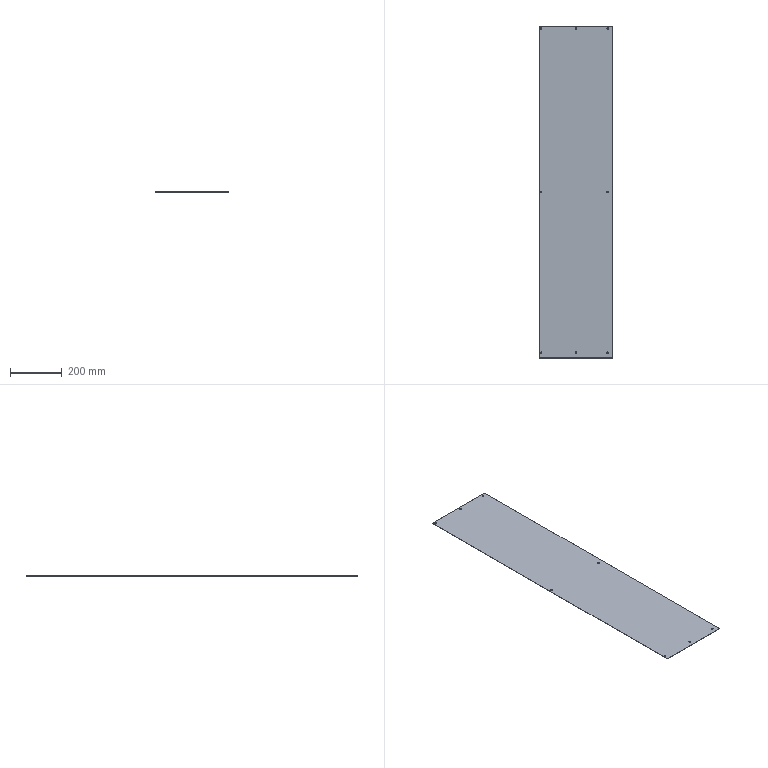Part | SolidWorks | features FlatPattern 1, HoleWzd 1, SMBaseFlange 1, SheetMetal 1 | 1 solid | 22 faces | box 285 x 1280 x 1.2 mm | volume 437432 mm3 | cylinder 16 | plane 6 | commonest cylinder face diameters 6.6 x16
STEP:
#1=CARTESIAN_POINT('',(-137.8,630.,-1.2));
#2=VERTEX_POINT('',#1);
#3=CARTESIAN_POINT('',(-131.2,630.,-1.2));
#4=VERTEX_POINT('',#3);
#5=CARTESIAN_POINT('',(-134.5,630.,-1.2));
#6=DIRECTION('',(0.,0.,1.));
#7=DIRECTION('',(1.,0.,0.));
#8=AXIS2_PLACEMENT_3D('',#5,#6,#7);
#9=CIRCLE('',#8,3.3);
#10=EDGE_CURVE('',#2,#4,#9,.T.);
#11=ORIENTED_EDGE('',*,*,#10,.F.);
#12=CARTESIAN_POINT('',(-137.8,630.,0.));
#13=VERTEX_POINT('',#12);
#14=CARTESIAN_POINT('',(-137.8,630.,0.));
#15=DIRECTION('',(0.,0.,1.));
#16=VECTOR('',#15,1000.);
#17=LINE('',#14,#16);
#18=EDGE_CURVE('',#2,#13,#17,.T.);
#19=ORIENTED_EDGE('',*,*,#18,.T.);
#20=CARTESIAN_POINT('',(-131.2,630.,0.));
#21=VERTEX_POINT('',#20);
#22=CARTESIAN_POINT('',(-134.5,630.,0.));
#23=DIRECTION('',(0.,0.,1.));
#24=DIRECTION('',(1.,0.,0.));
#25=AXIS2_PLACEMENT_3D('',#22,#23,#24);
#26=CIRCLE('',#25,3.3);
#27=EDGE_CURVE('',#13,#21,#26,.T.);
#28=ORIENTED_EDGE('',*,*,#27,.T.);
#29=CARTESIAN_POINT('',(-131.2,630.,0.));
#30=DIRECTION('',(0.,0.,1.));
#31=VECTOR('',#30,1000.);
#32=LINE('',#29,#31);
#33=EDGE_CURVE('',#4,#21,#32,.T.);
#34=ORIENTED_EDGE('',*,*,#33,.F.);
#35=EDGE_LOOP('',(#11,#19,#28,#34));
#36=FACE_OUTER_BOUND('',#35,.T.);
#37=CARTESIAN_POINT('',(-134.5,630.,0.));
#38=DIRECTION('',(0.,0.,1.));
#39=DIRECTION('',(1.,0.,0.));
#40=AXIS2_PLACEMENT_3D('',#37,#38,#39);
#41=CYLINDRICAL_SURFACE('',#40,3.3);
#42=ADVANCED_FACE('',(#36),#41,.F.);
#43=CARTESIAN_POINT('',(-137.8,0.,-1.2));
#44=VERTEX_POINT('',#43);
#45=CARTESIAN_POINT('',(-131.2,0.,-1.2));
#46=VERTEX_POINT('',#45);
#47=CARTESIAN_POINT('',(-134.5,0.,-1.2));
#48=DIRECTION('',(0.,0.,1.));
#49=DIRECTION('',(1.,0.,0.));
#50=AXIS2_PLACEMENT_3D('',#47,#48,#49);
#51=CIRCLE('',#50,3.3);
#52=EDGE_CURVE('',#44,#46,#51,.T.);
#53=ORIENTED_EDGE('',*,*,#52,.F.);
#54=CARTESIAN_POINT('',(-137.8,0.,0.));
#55=VERTEX_POINT('',#54);
#56=CARTESIAN_POINT('',(-137.8,0.,0.));
#57=DIRECTION('',(0.,0.,1.));
#58=VECTOR('',#57,1000.);
#59=LINE('',#56,#58);
#60=EDGE_CURVE('',#44,#55,#59,.T.);
#61=ORIENTED_EDGE('',*,*,#60,.T.);
#62=CARTESIAN_POINT('',(-131.2,0.,0.));
#63=VERTEX_POINT('',#62);
#64=CARTESIAN_POINT('',(-134.5,0.,0.));
#65=DIRECTION('',(0.,0.,1.));
#66=DIRECTION('',(1.,0.,0.));
#67=AXIS2_PLACEMENT_3D('',#64,#65,#66);
#68=CIRCLE('',#67,3.3);
#69=EDGE_CURVE('',#55,#63,#68,.T.);
#70=ORIENTED_EDGE('',*,*,#69,.T.);
#71=CARTESIAN_POINT('',(-131.2,0.,0.));
#72=DIRECTION('',(0.,0.,1.));
#73=VECTOR('',#72,1000.);
#74=LINE('',#71,#73);
#75=EDGE_CURVE('',#46,#63,#74,.T.);
#76=ORIENTED_EDGE('',*,*,#75,.F.);
#77=EDGE_LOOP('',(#53,#61,#70,#76));
#78=FACE_OUTER_BOUND('',#77,.T.);
#79=CARTESIAN_POINT('',(-134.5,0.,0.));
#80=DIRECTION('',(0.,0.,1.));
#81=DIRECTION('',(1.,0.,0.));
#82=AXIS2_PLACEMENT_3D('',#79,#80,#81);
#83=CYLINDRICAL_SURFACE('',#82,3.3);
#84=ADVANCED_FACE('',(#78),#83,.F.);
#85=CARTESIAN_POINT('',(-137.8,-620.,-1.2));
#86=VERTEX_POINT('',#85);
#87=CARTESIAN_POINT('',(-131.2,-620.,-1.2));
#88=VERTEX_POINT('',#87);
#89=CARTESIAN_POINT('',(-134.5,-620.,-1.2));
#90=DIRECTION('',(0.,0.,1.));
#91=DIRECTION('',(1.,0.,0.));
#92=AXIS2_PLACEMENT_3D('',#89,#90,#91);
#93=CIRCLE('',#92,3.3);
#94=EDGE_CURVE('',#86,#88,#93,.T.);
#95=ORIENTED_EDGE('',*,*,#94,.F.);
#96=CARTESIAN_POINT('',(-137.8,-620.,0.));
#97=VERTEX_POINT('',#96);
#98=CARTESIAN_POINT('',(-137.8,-620.,0.));
#99=DIRECTION('',(0.,0.,1.));
#100=VECTOR('',#99,1000.);
#101=LINE('',#98,#100);
#102=EDGE_CURVE('',#86,#97,#101,.T.);
#103=ORIENTED_EDGE('',*,*,#102,.T.);
#104=CARTESIAN_POINT('',(-131.2,-620.,0.));
#105=VERTEX_POINT('',#104);
#106=CARTESIAN_POINT('',(-134.5,-620.,0.));
#107=DIRECTION('',(0.,0.,1.));
#108=DIRECTION('',(1.,0.,0.));
#109=AXIS2_PLACEMENT_3D('',#106,#107,#108);
#110=CIRCLE('',#109,3.3);
#111=EDGE_CURVE('',#97,#105,#110,.T.);
#112=ORIENTED_EDGE('',*,*,#111,.T.);
#113=CARTESIAN_POINT('',(-131.2,-620.,0.));
#114=DIRECTION('',(0.,0.,1.));
#115=VECTOR('',#114,1000.);
#116=LINE('',#113,#115);
#117=EDGE_CURVE('',#88,#105,#116,.T.);
#118=ORIENTED_EDGE('',*,*,#117,.F.);
#119=EDGE_LOOP('',(#95,#103,#112,#118));
#120=FACE_OUTER_BOUND('',#119,.T.);
#121=CARTESIAN_POINT('',(-134.5,-620.,0.));
#122=DIRECTION('',(0.,0.,1.));
#123=DIRECTION('',(1.,0.,0.));
#124=AXIS2_PLACEMENT_3D('',#121,#122,#123);
#125=CYLINDRICAL_SURFACE('',#124,3.3);
#126=ADVANCED_FACE('',(#120),#125,.F.);
#127=CARTESIAN_POINT('',(-3.3,-620.,-1.2));
#128=VERTEX_POINT('',#127);
#129=CARTESIAN_POINT('',(3.3,-620.,-1.2));
#130=VERTEX_POINT('',#129);
#131=CARTESIAN_POINT('',(0.,-620.,-1.2));
#132=DIRECTION('',(0.,0.,1.));
#133=DIRECTION('',(1.,0.,0.));
#134=AXIS2_PLACEMENT_3D('',#131,#132,#133);
#135=CIRCLE('',#134,3.3);
#136=EDGE_CURVE('',#128,#130,#135,.T.);
#137=ORIENTED_EDGE('',*,*,#136,.F.);
#138=CARTESIAN_POINT('',(-3.3,-620.,0.));
#139=VERTEX_POINT('',#138);
#140=CARTESIAN_POINT('',(-3.3,-620.,0.));
#141=DIRECTION('',(0.,0.,1.));
#142=VECTOR('',#141,1000.);
#143=LINE('',#140,#142);
#144=EDGE_CURVE('',#128,#139,#143,.T.);
#145=ORIENTED_EDGE('',*,*,#144,.T.);
#146=CARTESIAN_POINT('',(3.3,-620.,0.));
#147=VERTEX_POINT('',#146);
#148=CARTESIAN_POINT('',(0.,-620.,0.));
#149=DIRECTION('',(0.,0.,1.));
#150=DIRECTION('',(1.,0.,0.));
#151=AXIS2_PLACEMENT_3D('',#148,#149,#150);
#152=CIRCLE('',#151,3.3);
#153=EDGE_CURVE('',#139,#147,#152,.T.);
#154=ORIENTED_EDGE('',*,*,#153,.T.);
#155=CARTESIAN_POINT('',(3.3,-620.,0.));
#156=DIRECTION('',(0.,0.,1.));
#157=VECTOR('',#156,1000.);
#158=LINE('',#155,#157);
#159=EDGE_CURVE('',#130,#147,#158,.T.);
#160=ORIENTED_EDGE('',*,*,#159,.F.);
#161=EDGE_LOOP('',(#137,#145,#154,#160));
#162=FACE_OUTER_BOUND('',#161,.T.);
#163=CARTESIAN_POINT('',(0.,-620.,0.));
#164=DIRECTION('',(0.,0.,1.));
#165=DIRECTION('',(1.,0.,0.));
#166=AXIS2_PLACEMENT_3D('',#163,#164,#165);
#167=CYLINDRICAL_SURFACE('',#166,3.3);
#168=ADVANCED_FACE('',(#162),#167,.F.);
#169=CARTESIAN_POINT('',(119.2,630.,-1.2));
#170=VERTEX_POINT('',#169);
#171=CARTESIAN_POINT('',(125.8,630.,-1.2));
#172=VERTEX_POINT('',#171);
#173=CARTESIAN_POINT('',(122.5,630.,-1.2));
#174=DIRECTION('',(0.,0.,1.));
#175=DIRECTION('',(1.,0.,0.));
#176=AXIS2_PLACEMENT_3D('',#173,#174,#175);
#177=CIRCLE('',#176,3.3);
#178=EDGE_CURVE('',#170,#172,#177,.T.);
#179=ORIENTED_EDGE('',*,*,#178,.F.);
#180=CARTESIAN_POINT('',(119.2,630.,0.));
#181=VERTEX_POINT('',#180);
#182=CARTESIAN_POINT('',(119.2,630.,0.));
#183=DIRECTION('',(0.,0.,1.));
#184=VECTOR('',#183,1000.);
#185=LINE('',#182,#184);
#186=EDGE_CURVE('',#170,#181,#185,.T.);
#187=ORIENTED_EDGE('',*,*,#186,.T.);
#188=CARTESIAN_POINT('',(125.8,630.,0.));
#189=VERTEX_POINT('',#188);
#190=CARTESIAN_POINT('',(122.5,630.,0.));
#191=DIRECTION('',(0.,0.,1.));
#192=DIRECTION('',(1.,0.,0.));
#193=AXIS2_PLACEMENT_3D('',#190,#191,#192);
#194=CIRCLE('',#193,3.3);
#195=EDGE_CURVE('',#181,#189,#194,.T.);
#196=ORIENTED_EDGE('',*,*,#195,.T.);
#197=CARTESIAN_POINT('',(125.8,630.,0.));
#198=DIRECTION('',(0.,0.,1.));
#199=VECTOR('',#198,1000.);
#200=LINE('',#197,#199);
#201=EDGE_CURVE('',#172,#189,#200,.T.);
#202=ORIENTED_EDGE('',*,*,#201,.F.);
#203=EDGE_LOOP('',(#179,#187,#196,#202));
#204=FACE_OUTER_BOUND('',#203,.T.);
#205=CARTESIAN_POINT('',(122.5,630.,0.));
#206=DIRECTION('',(0.,0.,1.));
#207=DIRECTION('',(1.,0.,0.));
#208=AXIS2_PLACEMENT_3D('',#205,#206,#207);
#209=CYLINDRICAL_SURFACE('',#208,3.3);
#210=ADVANCED_FACE('',(#204),#209,.F.);
#211=CARTESIAN_POINT('',(119.2,0.,-1.2));
#212=VERTEX_POINT('',#211);
#213=CARTESIAN_POINT('',(125.8,0.,-1.2));
#214=VERTEX_POINT('',#213);
#215=CARTESIAN_POINT('',(122.5,0.,-1.2));
#216=DIRECTION('',(0.,0.,1.));
#217=DIRECTION('',(1.,0.,0.));
#218=AXIS2_PLACEMENT_3D('',#215,#216,#217);
#219=CIRCLE('',#218,3.3);
#220=EDGE_CURVE('',#212,#214,#219,.T.);
#221=ORIENTED_EDGE('',*,*,#220,.F.);
#222=CARTESIAN_POINT('',(119.2,0.,0.));
#223=VERTEX_POINT('',#222);
#224=CARTESIAN_POINT('',(119.2,0.,0.));
#225=DIRECTION('',(0.,0.,1.));
#226=VECTOR('',#225,1000.);
#227=LINE('',#224,#226);
#228=EDGE_CURVE('',#212,#223,#227,.T.);
#229=ORIENTED_EDGE('',*,*,#228,.T.);
#230=CARTESIAN_POINT('',(125.8,0.,0.));
#231=VERTEX_POINT('',#230);
#232=CARTESIAN_POINT('',(122.5,0.,0.));
#233=DIRECTION('',(0.,0.,1.));
#234=DIRECTION('',(1.,0.,0.));
#235=AXIS2_PLACEMENT_3D('',#232,#233,#234);
#236=CIRCLE('',#235,3.3);
#237=EDGE_CURVE('',#223,#231,#236,.T.);
#238=ORIENTED_EDGE('',*,*,#237,.T.);
#239=CARTESIAN_POINT('',(125.8,0.,0.));
#240=DIRECTION('',(0.,0.,1.));
#241=VECTOR('',#240,1000.);
#242=LINE('',#239,#241);
#243=EDGE_CURVE('',#214,#231,#242,.T.);
#244=ORIENTED_EDGE('',*,*,#243,.F.);
#245=EDGE_LOOP('',(#221,#229,#238,#244));
#246=FACE_OUTER_BOUND('',#245,.T.);
#247=CARTESIAN_POINT('',(122.5,0.,0.));
#248=DIRECTION('',(0.,0.,1.));
#249=DIRECTION('',(1.,0.,0.));
#250=AXIS2_PLACEMENT_3D('',#247,#248,#249);
#251=CYLINDRICAL_SURFACE('',#250,3.3);
#252=ADVANCED_FACE('',(#246),#251,.F.);
#253=CARTESIAN_POINT('',(119.2,-620.,-1.2));
#254=VERTEX_POINT('',#253);
#255=CARTESIAN_POINT('',(125.8,-620.,-1.2));
#256=VERTEX_POINT('',#255);
#257=CARTESIAN_POINT('',(122.5,-620.,-1.2));
#258=DIRECTION('',(0.,0.,1.));
#259=DIRECTION('',(1.,0.,0.));
#260=AXIS2_PLACEMENT_3D('',#257,#258,#259);
#261=CIRCLE('',#260,3.3);
#262=EDGE_CURVE('',#254,#256,#261,.T.);
#263=ORIENTED_EDGE('',*,*,#262,.F.);
#264=CARTESIAN_POINT('',(119.2,-620.,0.));
#265=VERTEX_POINT('',#264);
#266=CARTESIAN_POINT('',(119.2,-620.,0.));
#267=DIRECTION('',(0.,0.,1.));
#268=VECTOR('',#267,1000.);
#269=LINE('',#266,#268);
#270=EDGE_CURVE('',#254,#265,#269,.T.);
#271=ORIENTED_EDGE('',*,*,#270,.T.);
#272=CARTESIAN_POINT('',(125.8,-620.,0.));
#273=VERTEX_POINT('',#272);
#274=CARTESIAN_POINT('',(122.5,-620.,0.));
#275=DIRECTION('',(0.,0.,1.));
#276=DIRECTION('',(1.,0.,0.));
#277=AXIS2_PLACEMENT_3D('',#274,#275,#276);
#278=CIRCLE('',#277,3.3);
#279=EDGE_CURVE('',#265,#273,#278,.T.);
#280=ORIENTED_EDGE('',*,*,#279,.T.);
#281=CARTESIAN_POINT('',(125.8,-620.,0.));
#282=DIRECTION('',(0.,0.,1.));
#283=VECTOR('',#282,1000.);
#284=LINE('',#281,#283);
#285=EDGE_CURVE('',#256,#273,#284,.T.);
#286=ORIENTED_EDGE('',*,*,#285,.F.);
#287=EDGE_LOOP('',(#263,#271,#280,#286));
#288=FACE_OUTER_BOUND('',#287,.T.);
#289=CARTESIAN_POINT('',(122.5,-620.,0.));
#290=DIRECTION('',(0.,0.,1.));
#291=DIRECTION('',(1.,0.,0.));
#292=AXIS2_PLACEMENT_3D('',#289,#290,#291);
#293=CYLINDRICAL_SURFACE('',#292,3.3);
#294=ADVANCED_FACE('',(#288),#293,.F.);
#295=CARTESIAN_POINT('',(-3.3,630.,-1.2));
#296=VERTEX_POINT('',#295);
#297=CARTESIAN_POINT('',(3.3,630.,-1.2));
#298=VERTEX_POINT('',#297);
#299=CARTESIAN_POINT('',(0.,630.,-1.2));
#300=DIRECTION('',(0.,0.,1.));
#301=DIRECTION('',(1.,0.,0.));
#302=AXIS2_PLACEMENT_3D('',#299,#300,#301);
#303=CIRCLE('',#302,3.3);
#304=EDGE_CURVE('',#296,#298,#303,.T.);
#305=ORIENTED_EDGE('',*,*,#304,.F.);
#306=CARTESIAN_POINT('',(-3.3,630.,0.));
#307=VERTEX_POINT('',#306);
#308=CARTESIAN_POINT('',(-3.3,630.,0.));
#309=DIRECTION('',(0.,0.,1.));
#310=VECTOR('',#309,1000.);
#311=LINE('',#308,#310);
#312=EDGE_CURVE('',#296,#307,#311,.T.);
#313=ORIENTED_EDGE('',*,*,#312,.T.);
#314=CARTESIAN_POINT('',(3.3,630.,0.));
#315=VERTEX_POINT('',#314);
#316=CARTESIAN_POINT('',(0.,630.,0.));
#317=DIRECTION('',(0.,0.,1.));
#318=DIRECTION('',(1.,0.,0.));
#319=AXIS2_PLACEMENT_3D('',#316,#317,#318);
#320=CIRCLE('',#319,3.3);
#321=EDGE_CURVE('',#307,#315,#320,.T.);
#322=ORIENTED_EDGE('',*,*,#321,.T.);
#323=CARTESIAN_POINT('',(3.3,630.,0.));
#324=DIRECTION('',(0.,0.,1.));
#325=VECTOR('',#324,1000.);
#326=LINE('',#323,#325);
#327=EDGE_CURVE('',#298,#315,#326,.T.);
#328=ORIENTED_EDGE('',*,*,#327,.F.);
#329=EDGE_LOOP('',(#305,#313,#322,#328));
#330=FACE_OUTER_BOUND('',#329,.T.);
#331=CARTESIAN_POINT('',(0.,630.,0.));
#332=DIRECTION('',(0.,0.,1.));
#333=DIRECTION('',(1.,0.,0.));
#334=AXIS2_PLACEMENT_3D('',#331,#332,#333);
#335=CYLINDRICAL_SURFACE('',#334,3.3);
#336=ADVANCED_FACE('',(#330),#335,.F.);
#337=CARTESIAN_POINT('',(142.5,-640.,0.));
#338=VERTEX_POINT('',#337);
#339=CARTESIAN_POINT('',(142.5,640.,0.));
#340=VERTEX_POINT('',#339);
#341=CARTESIAN_POINT('',(142.5,640.,0.));
#342=DIRECTION('',(0.,1.,0.));
#343=VECTOR('',#342,1000.);
#344=LINE('',#341,#343);
#345=EDGE_CURVE('',#338,#340,#344,.T.);
#346=ORIENTED_EDGE('',*,*,#345,.F.);
#347=CARTESIAN_POINT('',(142.5,-640.,-1.2));
#348=VERTEX_POINT('',#347);
#349=CARTESIAN_POINT('',(142.5,-640.,-1.2));
#350=DIRECTION('',(0.,0.,1.));
#351=VECTOR('',#350,1000.);
#352=LINE('',#349,#351);
#353=EDGE_CURVE('',#348,#338,#352,.T.);
#354=ORIENTED_EDGE('',*,*,#353,.F.);
#355=CARTESIAN_POINT('',(142.5,640.,-1.2));
#356=VERTEX_POINT('',#355);
#357=CARTESIAN_POINT('',(142.5,640.,-1.2));
#358=DIRECTION('',(0.,1.,0.));
#359=VECTOR('',#358,1000.);
#360=LINE('',#357,#359);
#361=EDGE_CURVE('',#348,#356,#360,.T.);
#362=ORIENTED_EDGE('',*,*,#361,.T.);
#363=CARTESIAN_POINT('',(142.5,640.,-1.2));
#364=DIRECTION('',(0.,0.,1.));
#365=VECTOR('',#364,1000.);
#366=LINE('',#363,#365);
#367=EDGE_CURVE('',#356,#340,#366,.T.);
#368=ORIENTED_EDGE('',*,*,#367,.T.);
#369=EDGE_LOOP('',(#346,#354,#362,#368));
#370=FACE_OUTER_BOUND('',#369,.T.);
#371=CARTESIAN_POINT('',(142.5,640.,-1.2));
#372=DIRECTION('',(1.,0.,0.));
#373=DIRECTION('',(0.,1.,0.));
#374=AXIS2_PLACEMENT_3D('',#371,#372,#373);
#375=PLANE('',#374);
#376=ADVANCED_FACE('',(#370),#375,.T.);
#377=CARTESIAN_POINT('',(-142.5,-640.,0.));
#378=VERTEX_POINT('',#377);
#379=CARTESIAN_POINT('',(-142.5,-640.,0.));
#380=DIRECTION('',(1.,0.,0.));
#381=VECTOR('',#380,1000.);
#382=LINE('',#379,#381);
#383=EDGE_CURVE('',#378,#338,#382,.T.);
#384=ORIENTED_EDGE('',*,*,#383,.F.);
#385=CARTESIAN_POINT('',(-142.5,-640.,-1.2));
#386=VERTEX_POINT('',#385);
#387=CARTESIAN_POINT('',(-142.5,-640.,-1.2));
#388=DIRECTION('',(0.,0.,1.));
#389=VECTOR('',#388,1000.);
#390=LINE('',#387,#389);
#391=EDGE_CURVE('',#386,#378,#390,.T.);
#392=ORIENTED_EDGE('',*,*,#391,.F.);
#393=CARTESIAN_POINT('',(-142.5,-640.,-1.2));
#394=DIRECTION('',(1.,0.,0.));
#395=VECTOR('',#394,1000.);
#396=LINE('',#393,#395);
#397=EDGE_CURVE('',#386,#348,#396,.T.);
#398=ORIENTED_EDGE('',*,*,#397,.T.);
#399=ORIENTED_EDGE('',*,*,#353,.T.);
#400=EDGE_LOOP('',(#384,#392,#398,#399));
#401=FACE_OUTER_BOUND('',#400,.T.);
#402=CARTESIAN_POINT('',(-142.5,-640.,-1.2));
#403=DIRECTION('',(0.,-1.,0.));
#404=DIRECTION('',(0.,0.,-1.));
#405=AXIS2_PLACEMENT_3D('',#402,#403,#404);
#406=PLANE('',#405);
#407=ADVANCED_FACE('',(#401),#406,.T.);
#408=CARTESIAN_POINT('',(-142.5,640.,0.));
#409=VERTEX_POINT('',#408);
#410=CARTESIAN_POINT('',(-142.5,640.,0.));
#411=DIRECTION('',(0.,-1.,0.));
#412=VECTOR('',#411,1000.);
#413=LINE('',#410,#412);
#414=EDGE_CURVE('',#409,#378,#413,.T.);
#415=ORIENTED_EDGE('',*,*,#414,.F.);
#416=CARTESIAN_POINT('',(-142.5,640.,-1.2));
#417=VERTEX_POINT('',#416);
#418=CARTESIAN_POINT('',(-142.5,640.,-1.2));
#419=DIRECTION('',(0.,0.,1.));
#420=VECTOR('',#419,1000.);
#421=LINE('',#418,#420);
#422=EDGE_CURVE('',#417,#409,#421,.T.);
#423=ORIENTED_EDGE('',*,*,#422,.F.);
#424=CARTESIAN_POINT('',(-142.5,640.,-1.2));
#425=DIRECTION('',(0.,-1.,0.));
#426=VECTOR('',#425,1000.);
#427=LINE('',#424,#426);
#428=EDGE_CURVE('',#417,#386,#427,.T.);
#429=ORIENTED_EDGE('',*,*,#428,.T.);
#430=ORIENTED_EDGE('',*,*,#391,.T.);
#431=EDGE_LOOP('',(#415,#423,#429,#430));
#432=FACE_OUTER_BOUND('',#431,.T.);
#433=CARTESIAN_POINT('',(-142.5,640.,-1.2));
#434=DIRECTION('',(-1.,0.,0.));
#435=DIRECTION('',(0.,-1.,0.));
#436=AXIS2_PLACEMENT_3D('',#433,#434,#435);
#437=PLANE('',#436);
#438=ADVANCED_FACE('',(#432),#437,.T.);
#439=CARTESIAN_POINT('',(-142.5,640.,0.));
#440=DIRECTION('',(-1.,0.,0.));
#441=VECTOR('',#440,1000.);
#442=LINE('',#439,#441);
#443=EDGE_CURVE('',#340,#409,#442,.T.);
#444=ORIENTED_EDGE('',*,*,#443,.F.);
#445=ORIENTED_EDGE('',*,*,#367,.F.);
#446=CARTESIAN_POINT('',(-142.5,640.,-1.2));
#447=DIRECTION('',(-1.,0.,0.));
#448=VECTOR('',#447,1000.);
#449=LINE('',#446,#448);
#450=EDGE_CURVE('',#356,#417,#449,.T.);
#451=ORIENTED_EDGE('',*,*,#450,.T.);
#452=ORIENTED_EDGE('',*,*,#422,.T.);
#453=EDGE_LOOP('',(#444,#445,#451,#452));
#454=FACE_OUTER_BOUND('',#453,.T.);
#455=CARTESIAN_POINT('',(-142.5,640.,-1.2));
#456=DIRECTION('',(0.,1.,0.));
#457=DIRECTION('',(0.,0.,1.));
#458=AXIS2_PLACEMENT_3D('',#455,#456,#457);
#459=PLANE('',#458);
#460=ADVANCED_FACE('',(#454),#459,.T.);
#461=CARTESIAN_POINT('',(-134.5,630.,-1.2));
#462=DIRECTION('',(0.,0.,1.));
#463=DIRECTION('',(1.,0.,0.));
#464=AXIS2_PLACEMENT_3D('',#461,#462,#463);
#465=CIRCLE('',#464,3.3);
#466=EDGE_CURVE('',#4,#2,#465,.T.);
#467=ORIENTED_EDGE('',*,*,#466,.T.);
#468=ORIENTED_EDGE('',*,*,#10,.T.);
#469=EDGE_LOOP('',(#467,#468));
#470=FACE_BOUND('',#469,.T.);
#471=CARTESIAN_POINT('',(-134.5,0.,-1.2));
#472=DIRECTION('',(0.,0.,1.));
#473=DIRECTION('',(1.,0.,0.));
#474=AXIS2_PLACEMENT_3D('',#471,#472,#473);
#475=CIRCLE('',#474,3.3);
#476=EDGE_CURVE('',#46,#44,#475,.T.);
#477=ORIENTED_EDGE('',*,*,#476,.T.);
#478=ORIENTED_EDGE('',*,*,#52,.T.);
#479=EDGE_LOOP('',(#477,#478));
#480=FACE_BOUND('',#479,.T.);
#481=CARTESIAN_POINT('',(-134.5,-620.,-1.2));
#482=DIRECTION('',(0.,0.,1.));
#483=DIRECTION('',(1.,0.,0.));
#484=AXIS2_PLACEMENT_3D('',#481,#482,#483);
#485=CIRCLE('',#484,3.3);
#486=EDGE_CURVE('',#88,#86,#485,.T.);
#487=ORIENTED_EDGE('',*,*,#486,.T.);
#488=ORIENTED_EDGE('',*,*,#94,.T.);
#489=EDGE_LOOP('',(#487,#488));
#490=FACE_BOUND('',#489,.T.);
#491=CARTESIAN_POINT('',(0.,-620.,-1.2));
#492=DIRECTION('',(0.,0.,1.));
#493=DIRECTION('',(1.,0.,0.));
#494=AXIS2_PLACEMENT_3D('',#491,#492,#493);
#495=CIRCLE('',#494,3.3);
#496=EDGE_CURVE('',#130,#128,#495,.T.);
#497=ORIENTED_EDGE('',*,*,#496,.T.);
#498=ORIENTED_EDGE('',*,*,#136,.T.);
#499=EDGE_LOOP('',(#497,#498));
#500=FACE_BOUND('',#499,.T.);
#501=CARTESIAN_POINT('',(122.5,630.,-1.2));
#502=DIRECTION('',(0.,0.,1.));
#503=DIRECTION('',(1.,0.,0.));
#504=AXIS2_PLACEMENT_3D('',#501,#502,#503);
#505=CIRCLE('',#504,3.3);
#506=EDGE_CURVE('',#172,#170,#505,.T.);
#507=ORIENTED_EDGE('',*,*,#506,.T.);
#508=ORIENTED_EDGE('',*,*,#178,.T.);
#509=EDGE_LOOP('',(#507,#508));
#510=FACE_BOUND('',#509,.T.);
#511=CARTESIAN_POINT('',(122.5,0.,-1.2));
#512=DIRECTION('',(0.,0.,1.));
#513=DIRECTION('',(1.,0.,0.));
#514=AXIS2_PLACEMENT_3D('',#511,#512,#513);
#515=CIRCLE('',#514,3.3);
#516=EDGE_CURVE('',#214,#212,#515,.T.);
#517=ORIENTED_EDGE('',*,*,#516,.T.);
#518=ORIENTED_EDGE('',*,*,#220,.T.);
#519=EDGE_LOOP('',(#517,#518));
#520=FACE_BOUND('',#519,.T.);
#521=CARTESIAN_POINT('',(122.5,-620.,-1.2));
#522=DIRECTION('',(0.,0.,1.));
#523=DIRECTION('',(1.,0.,0.));
#524=AXIS2_PLACEMENT_3D('',#521,#522,#523);
#525=CIRCLE('',#524,3.3);
#526=EDGE_CURVE('',#256,#254,#525,.T.);
#527=ORIENTED_EDGE('',*,*,#526,.T.);
#528=ORIENTED_EDGE('',*,*,#262,.T.);
#529=EDGE_LOOP('',(#527,#528));
#530=FACE_BOUND('',#529,.T.);
#531=CARTESIAN_POINT('',(0.,630.,-1.2));
#532=DIRECTION('',(0.,0.,1.));
#533=DIRECTION('',(1.,0.,0.));
#534=AXIS2_PLACEMENT_3D('',#531,#532,#533);
#535=CIRCLE('',#534,3.3);
#536=EDGE_CURVE('',#298,#296,#535,.T.);
#537=ORIENTED_EDGE('',*,*,#536,.T.);
#538=ORIENTED_EDGE('',*,*,#304,.T.);
#539=EDGE_LOOP('',(#537,#538));
#540=FACE_BOUND('',#539,.T.);
#541=ORIENTED_EDGE('',*,*,#361,.F.);
#542=ORIENTED_EDGE('',*,*,#397,.F.);
#543=ORIENTED_EDGE('',*,*,#428,.F.);
#544=ORIENTED_EDGE('',*,*,#450,.F.);
#545=EDGE_LOOP('',(#541,#542,#543,#544));
#546=FACE_OUTER_BOUND('',#545,.T.);
#547=CARTESIAN_POINT('',(0.,0.,-1.2));
#548=DIRECTION('',(0.,0.,1.));
#549=DIRECTION('',(1.,0.,0.));
#550=AXIS2_PLACEMENT_3D('',#547,#548,#549);
#551=PLANE('',#550);
#552=ADVANCED_FACE('',(#470,#480,#490,#500,#510,#520,#530,#540,#546),#551,.F.);
#553=CARTESIAN_POINT('',(-134.5,630.,0.));
#554=DIRECTION('',(0.,0.,1.));
#555=DIRECTION('',(1.,0.,0.));
#556=AXIS2_PLACEMENT_3D('',#553,#554,#555);
#557=CIRCLE('',#556,3.3);
#558=EDGE_CURVE('',#21,#13,#557,.T.);
#559=ORIENTED_EDGE('',*,*,#558,.F.);
#560=ORIENTED_EDGE('',*,*,#27,.F.);
#561=EDGE_LOOP('',(#559,#560));
#562=FACE_BOUND('',#561,.T.);
#563=CARTESIAN_POINT('',(-134.5,0.,0.));
#564=DIRECTION('',(0.,0.,1.));
#565=DIRECTION('',(1.,0.,0.));
#566=AXIS2_PLACEMENT_3D('',#563,#564,#565);
#567=CIRCLE('',#566,3.3);
#568=EDGE_CURVE('',#63,#55,#567,.T.);
#569=ORIENTED_EDGE('',*,*,#568,.F.);
#570=ORIENTED_EDGE('',*,*,#69,.F.);
#571=EDGE_LOOP('',(#569,#570));
#572=FACE_BOUND('',#571,.T.);
#573=CARTESIAN_POINT('',(-134.5,-620.,0.));
#574=DIRECTION('',(0.,0.,1.));
#575=DIRECTION('',(1.,0.,0.));
#576=AXIS2_PLACEMENT_3D('',#573,#574,#575);
#577=CIRCLE('',#576,3.3);
#578=EDGE_CURVE('',#105,#97,#577,.T.);
#579=ORIENTED_EDGE('',*,*,#578,.F.);
#580=ORIENTED_EDGE('',*,*,#111,.F.);
#581=EDGE_LOOP('',(#579,#580));
#582=FACE_BOUND('',#581,.T.);
#583=CARTESIAN_POINT('',(0.,-620.,0.));
#584=DIRECTION('',(0.,0.,1.));
#585=DIRECTION('',(1.,0.,0.));
#586=AXIS2_PLACEMENT_3D('',#583,#584,#585);
#587=CIRCLE('',#586,3.3);
#588=EDGE_CURVE('',#147,#139,#587,.T.);
#589=ORIENTED_EDGE('',*,*,#588,.F.);
#590=ORIENTED_EDGE('',*,*,#153,.F.);
#591=EDGE_LOOP('',(#589,#590));
#592=FACE_BOUND('',#591,.T.);
#593=CARTESIAN_POINT('',(122.5,630.,0.));
#594=DIRECTION('',(0.,0.,1.));
#595=DIRECTION('',(1.,0.,0.));
#596=AXIS2_PLACEMENT_3D('',#593,#594,#595);
#597=CIRCLE('',#596,3.3);
#598=EDGE_CURVE('',#189,#181,#597,.T.);
#599=ORIENTED_EDGE('',*,*,#598,.F.);
#600=ORIENTED_EDGE('',*,*,#195,.F.);
#601=EDGE_LOOP('',(#599,#600));
#602=FACE_BOUND('',#601,.T.);
#603=CARTESIAN_POINT('',(122.5,0.,0.));
#604=DIRECTION('',(0.,0.,1.));
#605=DIRECTION('',(1.,0.,0.));
#606=AXIS2_PLACEMENT_3D('',#603,#604,#605);
#607=CIRCLE('',#606,3.3);
#608=EDGE_CURVE('',#231,#223,#607,.T.);
#609=ORIENTED_EDGE('',*,*,#608,.F.);
#610=ORIENTED_EDGE('',*,*,#237,.F.);
#611=EDGE_LOOP('',(#609,#610));
#612=FACE_BOUND('',#611,.T.);
#613=CARTESIAN_POINT('',(122.5,-620.,0.));
#614=DIRECTION('',(0.,0.,1.));
#615=DIRECTION('',(1.,0.,0.));
#616=AXIS2_PLACEMENT_3D('',#613,#614,#615);
#617=CIRCLE('',#616,3.3);
#618=EDGE_CURVE('',#273,#265,#617,.T.);
#619=ORIENTED_EDGE('',*,*,#618,.F.);
#620=ORIENTED_EDGE('',*,*,#279,.F.);
#621=EDGE_LOOP('',(#619,#620));
#622=FACE_BOUND('',#621,.T.);
#623=CARTESIAN_POINT('',(0.,630.,0.));
#624=DIRECTION('',(0.,0.,1.));
#625=DIRECTION('',(1.,0.,0.));
#626=AXIS2_PLACEMENT_3D('',#623,#624,#625);
#627=CIRCLE('',#626,3.3);
#628=EDGE_CURVE('',#315,#307,#627,.T.);
#629=ORIENTED_EDGE('',*,*,#628,.F.);
#630=ORIENTED_EDGE('',*,*,#321,.F.);
#631=EDGE_LOOP('',(#629,#630));
#632=FACE_BOUND('',#631,.T.);
#633=ORIENTED_EDGE('',*,*,#345,.T.);
#634=ORIENTED_EDGE('',*,*,#443,.T.);
#635=ORIENTED_EDGE('',*,*,#414,.T.);
#636=ORIENTED_EDGE('',*,*,#383,.T.);
#637=EDGE_LOOP('',(#633,#634,#635,#636));
#638=FACE_OUTER_BOUND('',#637,.T.);
#639=CARTESIAN_POINT('',(0.,0.,0.));
#640=DIRECTION('',(0.,0.,1.));
#641=DIRECTION('',(1.,0.,0.));
#642=AXIS2_PLACEMENT_3D('',#639,#640,#641);
#643=PLANE('',#642);
#644=ADVANCED_FACE('',(#562,#572,#582,#592,#602,#612,#622,#632,#638),#643,.T.);
#645=ORIENTED_EDGE('',*,*,#312,.F.);
#646=ORIENTED_EDGE('',*,*,#536,.F.);
#647=ORIENTED_EDGE('',*,*,#327,.T.);
#648=ORIENTED_EDGE('',*,*,#628,.T.);
#649=EDGE_LOOP('',(#645,#646,#647,#648));
#650=FACE_OUTER_BOUND('',#649,.T.);
#651=CARTESIAN_POINT('',(0.,630.,0.));
#652=DIRECTION('',(0.,0.,1.));
#653=DIRECTION('',(1.,0.,0.));
#654=AXIS2_PLACEMENT_3D('',#651,#652,#653);
#655=CYLINDRICAL_SURFACE('',#654,3.3);
#656=ADVANCED_FACE('',(#650),#655,.F.);
#657=ORIENTED_EDGE('',*,*,#270,.F.);
#658=ORIENTED_EDGE('',*,*,#526,.F.);
#659=ORIENTED_EDGE('',*,*,#285,.T.);
#660=ORIENTED_EDGE('',*,*,#618,.T.);
#661=EDGE_LOOP('',(#657,#658,#659,#660));
#662=FACE_OUTER_BOUND('',#661,.T.);
#663=CARTESIAN_POINT('',(122.5,-620.,0.));
#664=DIRECTION('',(0.,0.,1.));
#665=DIRECTION('',(1.,0.,0.));
#666=AXIS2_PLACEMENT_3D('',#663,#664,#665);
#667=CYLINDRICAL_SURFACE('',#666,3.3);
#668=ADVANCED_FACE('',(#662),#667,.F.);
#669=ORIENTED_EDGE('',*,*,#228,.F.);
#670=ORIENTED_EDGE('',*,*,#516,.F.);
#671=ORIENTED_EDGE('',*,*,#243,.T.);
#672=ORIENTED_EDGE('',*,*,#608,.T.);
#673=EDGE_LOOP('',(#669,#670,#671,#672));
#674=FACE_OUTER_BOUND('',#673,.T.);
#675=CARTESIAN_POINT('',(122.5,0.,0.));
#676=DIRECTION('',(0.,0.,1.));
#677=DIRECTION('',(1.,0.,0.));
#678=AXIS2_PLACEMENT_3D('',#675,#676,#677);
#679=CYLINDRICAL_SURFACE('',#678,3.3);
#680=ADVANCED_FACE('',(#674),#679,.F.);
#681=ORIENTED_EDGE('',*,*,#186,.F.);
#682=ORIENTED_EDGE('',*,*,#506,.F.);
#683=ORIENTED_EDGE('',*,*,#201,.T.);
#684=ORIENTED_EDGE('',*,*,#598,.T.);
#685=EDGE_LOOP('',(#681,#682,#683,#684));
#686=FACE_OUTER_BOUND('',#685,.T.);
#687=CARTESIAN_POINT('',(122.5,630.,0.));
#688=DIRECTION('',(0.,0.,1.));
#689=DIRECTION('',(1.,0.,0.));
#690=AXIS2_PLACEMENT_3D('',#687,#688,#689);
#691=CYLINDRICAL_SURFACE('',#690,3.3);
#692=ADVANCED_FACE('',(#686),#691,.F.);
#693=ORIENTED_EDGE('',*,*,#144,.F.);
#694=ORIENTED_EDGE('',*,*,#496,.F.);
#695=ORIENTED_EDGE('',*,*,#159,.T.);
#696=ORIENTED_EDGE('',*,*,#588,.T.);
#697=EDGE_LOOP('',(#693,#694,#695,#696));
#698=FACE_OUTER_BOUND('',#697,.T.);
#699=CARTESIAN_POINT('',(0.,-620.,0.));
#700=DIRECTION('',(0.,0.,1.));
#701=DIRECTION('',(1.,0.,0.));
#702=AXIS2_PLACEMENT_3D('',#699,#700,#701);
#703=CYLINDRICAL_SURFACE('',#702,3.3);
#704=ADVANCED_FACE('',(#698),#703,.F.);
#705=ORIENTED_EDGE('',*,*,#102,.F.);
#706=ORIENTED_EDGE('',*,*,#486,.F.);
#707=ORIENTED_EDGE('',*,*,#117,.T.);
#708=ORIENTED_EDGE('',*,*,#578,.T.);
#709=EDGE_LOOP('',(#705,#706,#707,#708));
#710=FACE_OUTER_BOUND('',#709,.T.);
#711=CARTESIAN_POINT('',(-134.5,-620.,0.));
#712=DIRECTION('',(0.,0.,1.));
#713=DIRECTION('',(1.,0.,0.));
#714=AXIS2_PLACEMENT_3D('',#711,#712,#713);
#715=CYLINDRICAL_SURFACE('',#714,3.3);
#716=ADVANCED_FACE('',(#710),#715,.F.);
#717=ORIENTED_EDGE('',*,*,#60,.F.);
#718=ORIENTED_EDGE('',*,*,#476,.F.);
#719=ORIENTED_EDGE('',*,*,#75,.T.);
#720=ORIENTED_EDGE('',*,*,#568,.T.);
#721=EDGE_LOOP('',(#717,#718,#719,#720));
#722=FACE_OUTER_BOUND('',#721,.T.);
#723=CARTESIAN_POINT('',(-134.5,0.,0.));
#724=DIRECTION('',(0.,0.,1.));
#725=DIRECTION('',(1.,0.,0.));
#726=AXIS2_PLACEMENT_3D('',#723,#724,#725);
#727=CYLINDRICAL_SURFACE('',#726,3.3);
#728=ADVANCED_FACE('',(#722),#727,.F.);
#729=ORIENTED_EDGE('',*,*,#18,.F.);
#730=ORIENTED_EDGE('',*,*,#466,.F.);
#731=ORIENTED_EDGE('',*,*,#33,.T.);
#732=ORIENTED_EDGE('',*,*,#558,.T.);
#733=EDGE_LOOP('',(#729,#730,#731,#732));
#734=FACE_OUTER_BOUND('',#733,.T.);
#735=CARTESIAN_POINT('',(-134.5,630.,0.));
#736=DIRECTION('',(0.,0.,1.));
#737=DIRECTION('',(1.,0.,0.));
#738=AXIS2_PLACEMENT_3D('',#735,#736,#737);
#739=CYLINDRICAL_SURFACE('',#738,3.3);
#740=ADVANCED_FACE('',(#734),#739,.F.);
#741=CLOSED_SHELL('',(#42,#84,#126,#168,#210,#252,#294,#336,#376,#407,#438,#460,#552,#644,#656,#668,#680,#692,#704,#716,#728,#740));
#742=MANIFOLD_SOLID_BREP('',#741);
#743=CARTESIAN_POINT('',(0.,0.,0.));
#744=DIRECTION('',(0.,0.,1.));
#745=DIRECTION('',(1.,0.,0.));
#746=AXIS2_PLACEMENT_3D('',#743,#744,#745);
#747=(LENGTH_UNIT()NAMED_UNIT(*)SI_UNIT(.MILLI.,.METRE.));
#748=UNCERTAINTY_MEASURE_WITH_UNIT(LENGTH_MEASURE(0.00001),#747,'','');
#749=(NAMED_UNIT(*)PLANE_ANGLE_UNIT()SI_UNIT($,.RADIAN.));
#750=(NAMED_UNIT(*)SI_UNIT($,.STERADIAN.)SOLID_ANGLE_UNIT());
#751=(GEOMETRIC_REPRESENTATION_CONTEXT(3)GLOBAL_UNCERTAINTY_ASSIGNED_CONTEXT((#748))GLOBAL_UNIT_ASSIGNED_CONTEXT((#747,#749,#750))REPRESENTATION_CONTEXT('',''));
#752=ADVANCED_BREP_SHAPE_REPRESENTATION('',(#742,#746),#751);